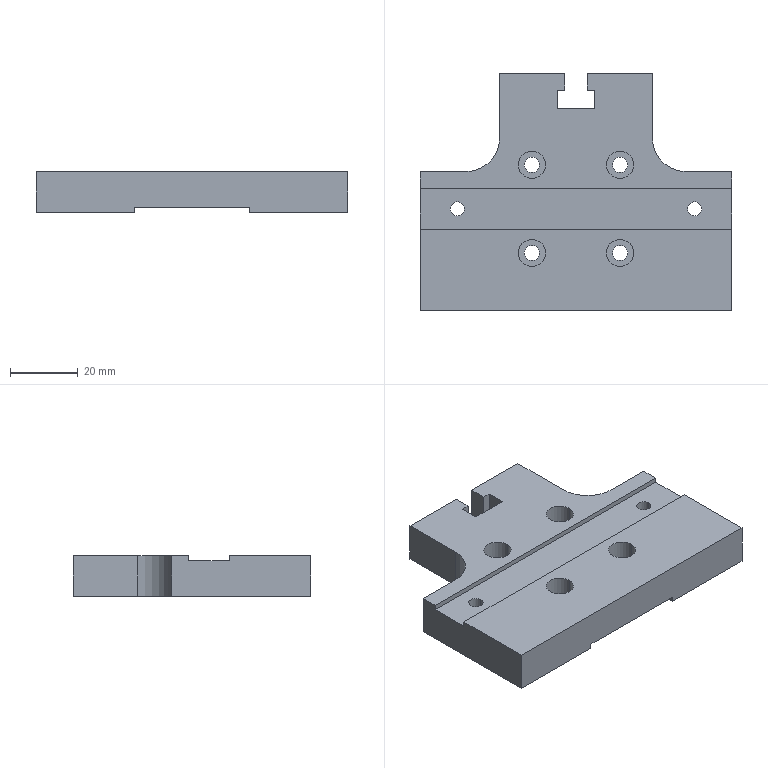Part | STEP file | 2098 Connecting plate A | 1 solid | 52 faces | box 92 x 70 x 12 mm | volume 53453 mm3 | plane 30 | cylinder 22 | commonest cylinder face diameters 4.5 x8 8 x8 4.2 x4 20 x2